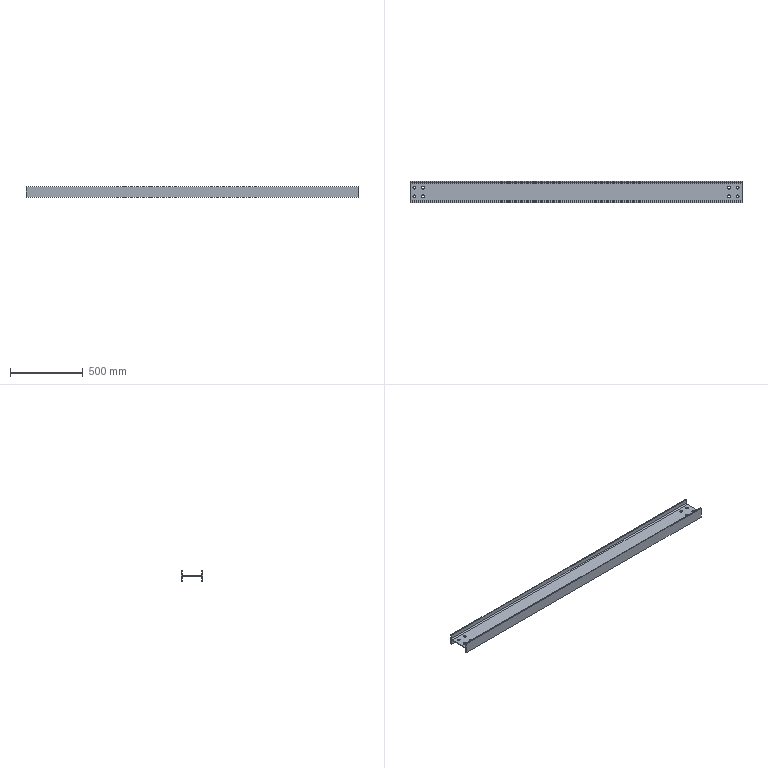Part | STEP file | 电柜辅梁2主体_Default<As Machined> | 1 solid | 34 faces | box 2280 x 150 x 75 mm | volume 4058318 mm3 | cylinder 20 | plane 14 | commonest cylinder face diameters 19 x16 16 x4